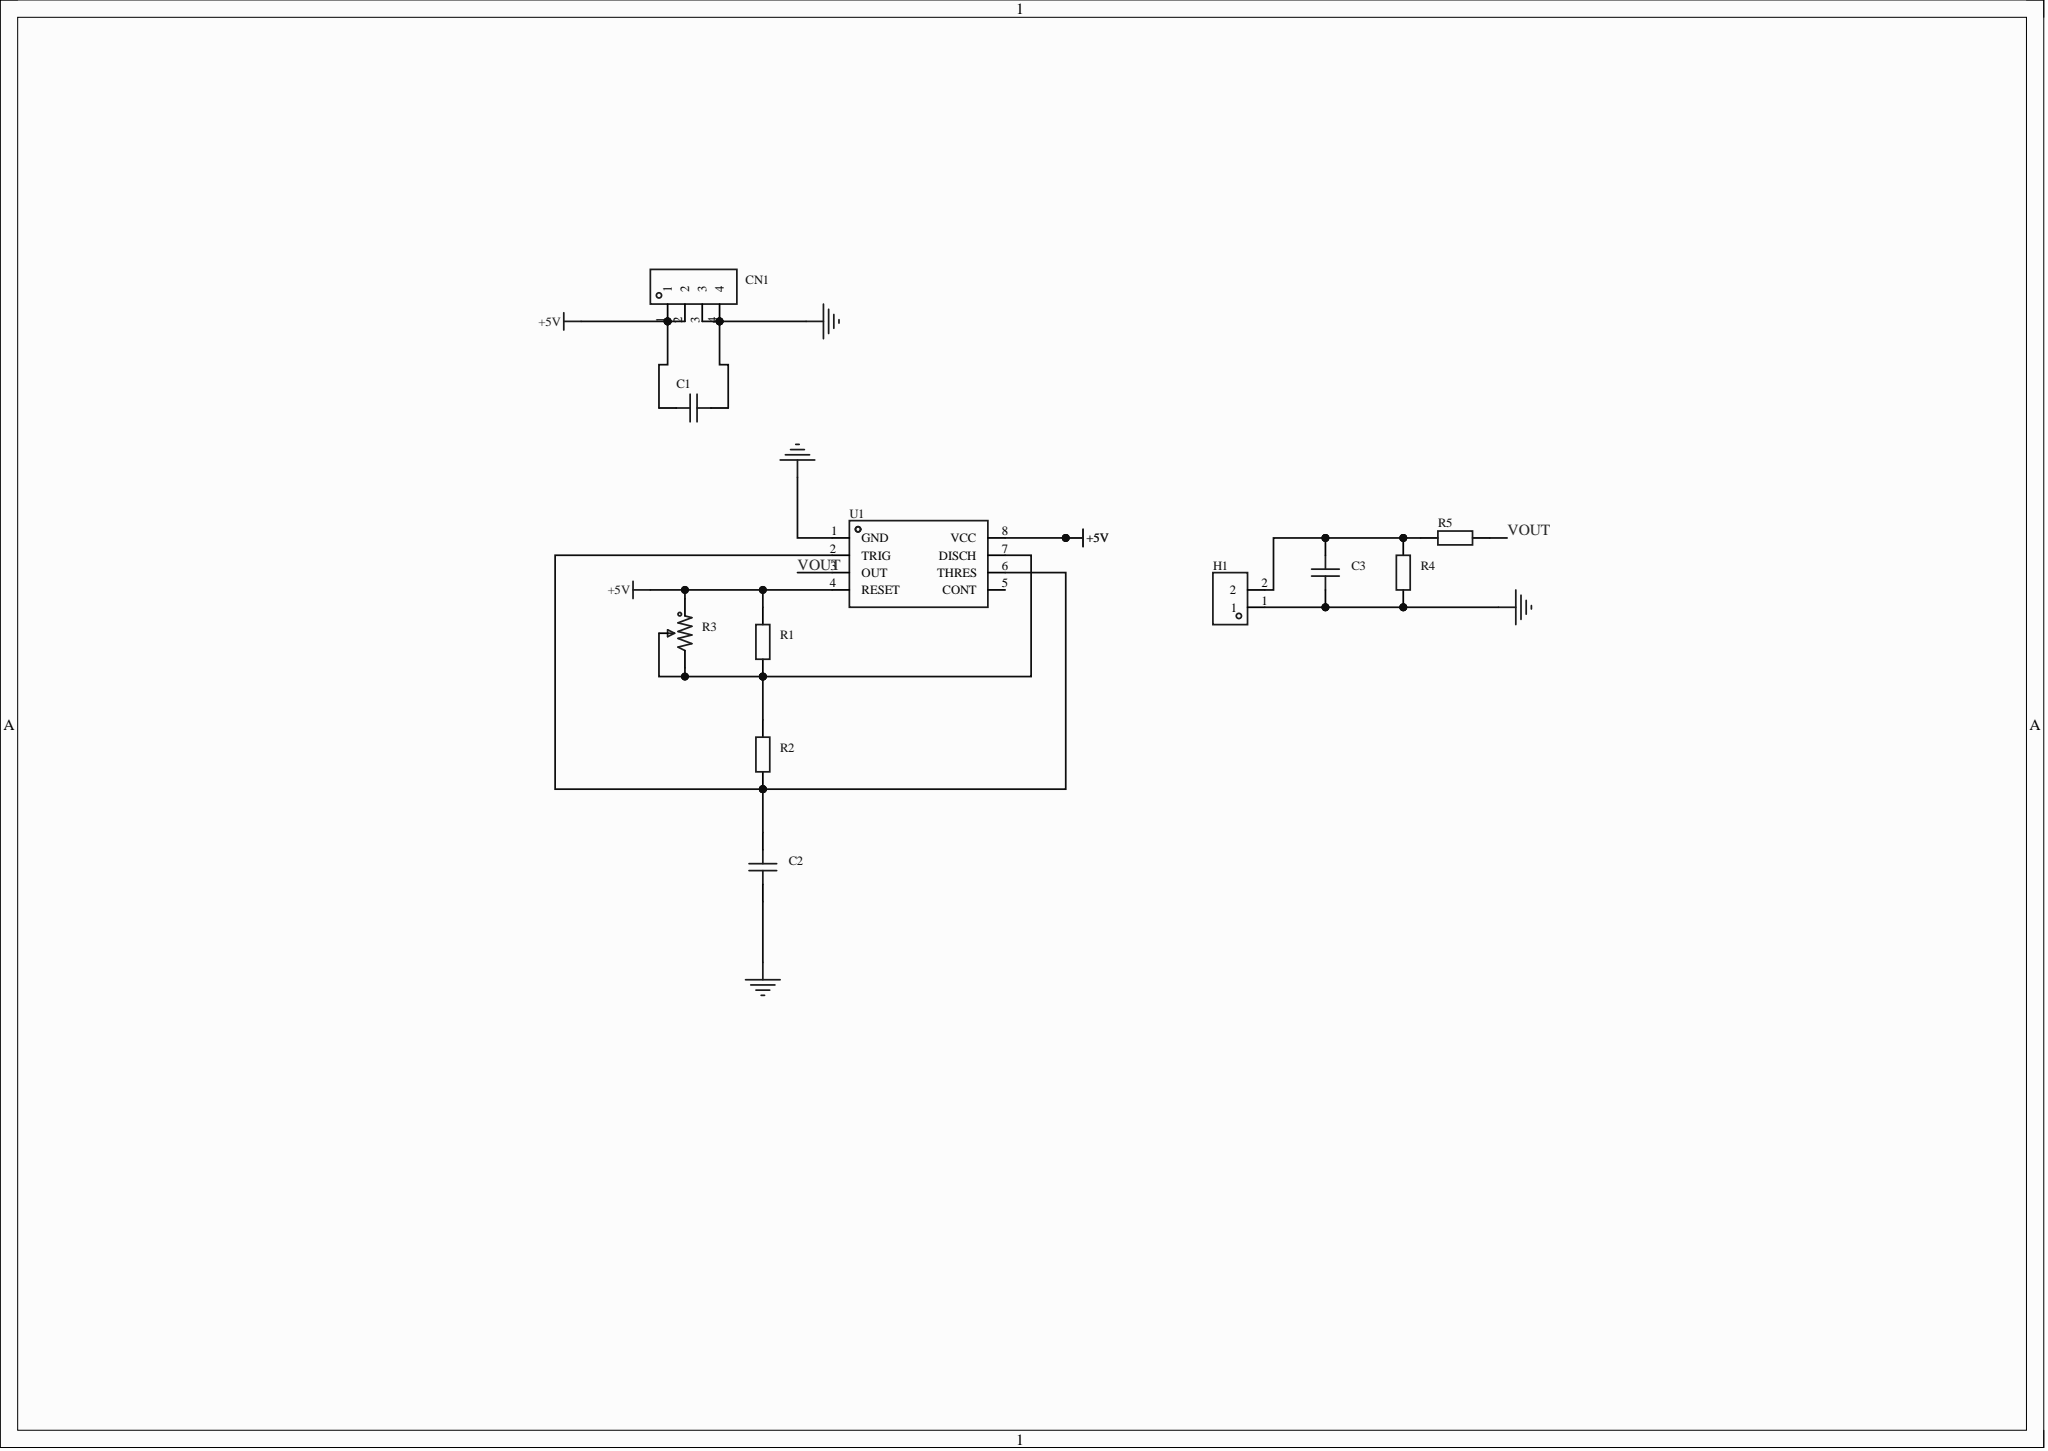Circuit board | Altium Designer | 11 parts | 6 nets
Bill of materials:
Comment,Description,Designator,Footprint,LibRef,Quantity
"1uF","Capacitance: 22uF; Tolerance: ±20%; Rated voltage: 35V; Dielectric (temperature coefficient): X5R;","C1","C0805","1uF","1"
"10nF","Capacitance: 22uF; Tolerance: ±20%; Rated voltage: 35V; Dielectric (temperature coefficient): X5R;","C2","C0805","10nF","1"
"200pF","Capacitance: 200pF; Tolerance: ±5%; Rated voltage: 50V; Dielectric (temperature coefficient): NP0;","C3","C0805","200pF","1"
"A2541WV-4P","Pin structure: 1x4P; Pitch: 2.54mm; Row spacing: -; Round/square pin: square pin; Mounting type: through-hole; Rows: single row; Total pins: 4P; Rated current: 3A; Rated voltage: 250V; Mating pin length: 6mm; Housing height: 2.54mm; Tail pin length: 3mm; Contact material: brass; Contact plating: gold; Operating temperature range: -40℃~+105℃; Color: black;","CN1","HDR-TH_4P-P2.54-V-M","A2541WV-4P","1"
"A2541WV-2P","Pin structure: 1x2P; Pitch: 2.54mm; Row spacing: -; Round/square pin: square pin; Mounting type: through-hole; Rows: single row; Total pins: 2P; Rated current: 3A; Rated voltage: 250V; Mating pin length: 6mm; Housing height: 2.54mm; Tail pin length: 3mm; Contact material: brass; Contact plating: gold; Operating temperature range: -40℃~+105℃; Color: black;","H1","HDR-TH_P2.54-H-M_A2541WV-2P","A2541WV-2P","1"
"5kO","Resistor type: thick film resistor; Resistance: 10kO; Tolerance: ±5%; Power: 125mW; Max working voltage: 150V; Temperature coefficient: ±100ppm/?;","R1","R0805","5kO","1"
"3kO","Resistor type: thick film resistor; Resistance: 10kO; Tolerance: ±5%; Power: 125mW; Max working voltage: 150V; Temperature coefficient: ±100ppm/?;","R2","R0805","3kO","1"
"5kO","Resistance: 10kO; Tolerance: ±10%;","R3","RES-ADJ-TH_3P-L10.0-W10.0-P2.50-L","5kO","1"
"10kO","Resistor type: thick film resistor; Resistance: 10kO; Tolerance: ±1%; Power: 125mW; Max working voltage: 150V; Temperature coefficient: ±100ppm/?;","R4, R5","R0805","10kO","2"
"100kHz","Frequency: 100kHz;","U1","SOP-8_L5.0-W4.0-P1.27-LS6.0-BL","100kHz","1"
Netlist (Protel format):
[
C1
C0805
1uF



]
[
C2
C0805
10nF



]
[
C3
C0805
200pF



]
[
CN1
HDR-TH_4P-P2.54-V-M
A2541WV-4P



]
[
H1
HDR-TH_P2.54-H-M_A2541WV-2P
A2541WV-2P



]
[
R1
R0805
5kO



]
[
R2
R0805
3kO



]
[
R3
RES-ADJ-TH_3P-L10.0-W10.0-P2.50-L
5kO



]
[
R4
R0805
10kO



]
[
R5
R0805
10kO



]
[
U1
SOP-8_L5.0-W4.0-P1.27-LS6.0-BL
100kHz



]
(
VOUT
R5-2
U1-3
)
(
NetR1_1
R1-1
R2-2
R3-2
R3-3
U1-7
)
(
NetC3_2
C3-2
H1-2
R4-2
R5-1
)
(
NetC2_2
C2-2
R2-1
U1-2
U1-6
)
(
GND
C1-1
C2-1
C3-1
CN1-3
CN1-4
H1-1
R4-1
U1-1
)
(
+5V
C1-2
CN1-1
CN1-2
R1-2
R3-1
U1-4
U1-8
)